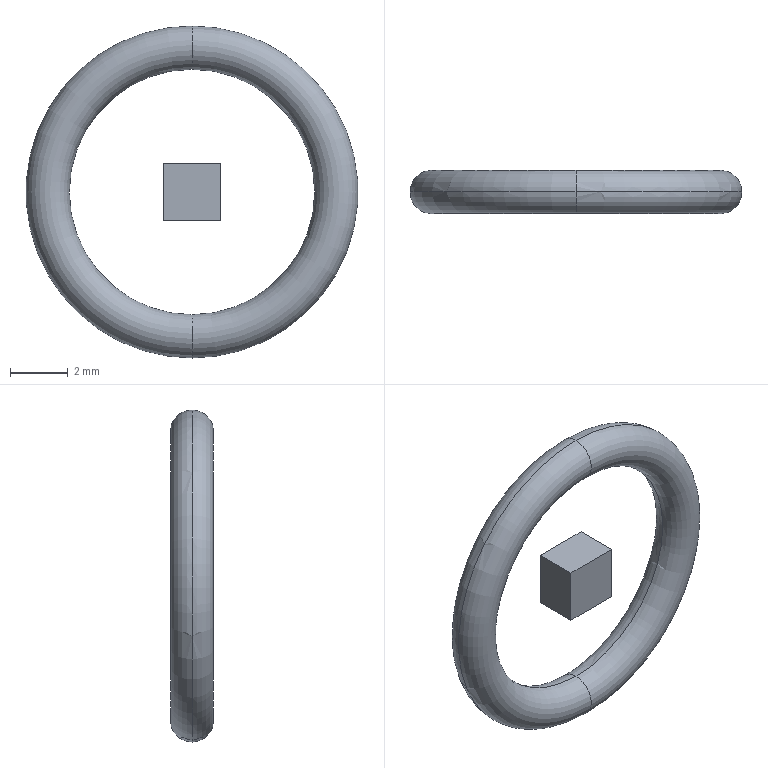Part | STEP file | O-ring ID 8.5 x 1.5 | 2 solids | 10 faces | box 11.5 x 1.5 x 11.5 mm | volume 61.517 mm3 | plane 6 | torus 4
STEP:
#1=CARTESIAN_POINT('',(0.,0.,0.));
#2=DIRECTION('',(0.,0.,1.));
#3=DIRECTION('',(1.,0.,0.));
#4=AXIS2_PLACEMENT_3D('',#1,#2,#3);
#5=CARTESIAN_POINT('',(0.,0.,5.75));
#6=VERTEX_POINT('',#5);
#7=CARTESIAN_POINT('',(0.,0.,4.25));
#8=VERTEX_POINT('',#7);
#9=CARTESIAN_POINT('',(0.,0.,5.));
#10=DIRECTION('',(1.,0.,0.));
#11=DIRECTION('',(0.,0.,-1.));
#12=AXIS2_PLACEMENT_3D('',#9,#10,#11);
#13=CIRCLE('',#12,0.75);
#14=CARTESIAN_POINT('',(0.,0.,0.));
#15=DIRECTION('',(0.,-1.,0.));
#16=DIRECTION('',(0.,0.,-1.));
#17=AXIS2_PLACEMENT_3D('',#14,#15,#16);
#18=TOROIDAL_SURFACE('',#17,5.,0.75);
#19=CARTESIAN_POINT('',(3.142,-3.142));
#20=DIRECTION('',(0.,1.));
#21=VECTOR('',#20,1.);
#22=LINE('',#19,#21);
#23=(GEOMETRIC_REPRESENTATION_CONTEXT(2)PARAMETRIC_REPRESENTATION_CONTEXT()REPRESENTATION_CONTEXT('',''));
#24=DEFINITIONAL_REPRESENTATION('',(#22),#23);
#25=PCURVE('',#18,#24);
#26=CARTESIAN_POINT('',(0.,0.,0.));
#27=DIRECTION('',(0.,-1.,0.));
#28=DIRECTION('',(0.,0.,-1.));
#29=AXIS2_PLACEMENT_3D('',#26,#27,#28);
#30=TOROIDAL_SURFACE('',#29,5.,0.75);
#31=CARTESIAN_POINT('',(3.142,-3.142));
#32=DIRECTION('',(0.,1.));
#33=VECTOR('',#32,1.);
#34=LINE('',#31,#33);
#35=(GEOMETRIC_REPRESENTATION_CONTEXT(2)PARAMETRIC_REPRESENTATION_CONTEXT()REPRESENTATION_CONTEXT('',''));
#36=DEFINITIONAL_REPRESENTATION('',(#34),#35);
#37=PCURVE('',#30,#36);
#38=SURFACE_CURVE('',#13,(#25,#37),.PCURVE_S1.);
#39=EDGE_CURVE('',#6,#8,#38,.T.);
#40=ORIENTED_EDGE('',*,*,#39,.F.);
#41=CARTESIAN_POINT('',(0.,0.,-5.75));
#42=VERTEX_POINT('',#41);
#43=CARTESIAN_POINT('',(0.,0.,0.));
#44=DIRECTION('',(0.,-1.,0.));
#45=DIRECTION('',(0.,0.,-1.));
#46=AXIS2_PLACEMENT_3D('',#43,#44,#45);
#47=CIRCLE('',#46,5.75);
#48=CARTESIAN_POINT('',(0.,0.));
#49=DIRECTION('',(1.,0.));
#50=VECTOR('',#49,1.);
#51=LINE('',#48,#50);
#52=(GEOMETRIC_REPRESENTATION_CONTEXT(2)PARAMETRIC_REPRESENTATION_CONTEXT()REPRESENTATION_CONTEXT('',''));
#53=DEFINITIONAL_REPRESENTATION('',(#51),#52);
#54=PCURVE('',#18,#53);
#55=CARTESIAN_POINT('',(0.,0.,0.));
#56=DIRECTION('',(0.,-1.,0.));
#57=DIRECTION('',(0.,0.,-1.));
#58=AXIS2_PLACEMENT_3D('',#55,#56,#57);
#59=TOROIDAL_SURFACE('',#58,5.,0.75);
#60=CARTESIAN_POINT('',(0.,6.283));
#61=DIRECTION('',(1.,0.));
#62=VECTOR('',#61,1.);
#63=LINE('',#60,#62);
#64=(GEOMETRIC_REPRESENTATION_CONTEXT(2)PARAMETRIC_REPRESENTATION_CONTEXT()REPRESENTATION_CONTEXT('',''));
#65=DEFINITIONAL_REPRESENTATION('',(#63),#64);
#66=PCURVE('',#59,#65);
#67=SURFACE_CURVE('',#47,(#54,#66),.PCURVE_S1.);
#68=EDGE_CURVE('',#6,#42,#67,.T.);
#69=ORIENTED_EDGE('',*,*,#68,.T.);
#70=CARTESIAN_POINT('',(0.,0.,-4.25));
#71=VERTEX_POINT('',#70);
#72=CARTESIAN_POINT('',(0.,0.,-5.));
#73=DIRECTION('',(-1.,0.,0.));
#74=DIRECTION('',(0.,0.,1.));
#75=AXIS2_PLACEMENT_3D('',#72,#73,#74);
#76=CIRCLE('',#75,0.75);
#77=CARTESIAN_POINT('',(6.283,-3.142));
#78=DIRECTION('',(0.,1.));
#79=VECTOR('',#78,1.);
#80=LINE('',#77,#79);
#81=(GEOMETRIC_REPRESENTATION_CONTEXT(2)PARAMETRIC_REPRESENTATION_CONTEXT()REPRESENTATION_CONTEXT('',''));
#82=DEFINITIONAL_REPRESENTATION('',(#80),#81);
#83=PCURVE('',#18,#82);
#84=CARTESIAN_POINT('',(0.,-3.142));
#85=DIRECTION('',(0.,1.));
#86=VECTOR('',#85,1.);
#87=LINE('',#84,#86);
#88=(GEOMETRIC_REPRESENTATION_CONTEXT(2)PARAMETRIC_REPRESENTATION_CONTEXT()REPRESENTATION_CONTEXT('',''));
#89=DEFINITIONAL_REPRESENTATION('',(#87),#88);
#90=PCURVE('',#30,#89);
#91=SURFACE_CURVE('',#76,(#83,#90),.PCURVE_S1.);
#92=EDGE_CURVE('',#42,#71,#91,.T.);
#93=ORIENTED_EDGE('',*,*,#92,.T.);
#94=CARTESIAN_POINT('',(0.,0.,0.));
#95=DIRECTION('',(0.,-1.,0.));
#96=DIRECTION('',(0.,0.,-1.));
#97=AXIS2_PLACEMENT_3D('',#94,#95,#96);
#98=CIRCLE('',#97,4.25);
#99=CARTESIAN_POINT('',(0.,3.142));
#100=DIRECTION('',(1.,0.));
#101=VECTOR('',#100,1.);
#102=LINE('',#99,#101);
#103=(GEOMETRIC_REPRESENTATION_CONTEXT(2)PARAMETRIC_REPRESENTATION_CONTEXT()REPRESENTATION_CONTEXT('',''));
#104=DEFINITIONAL_REPRESENTATION('',(#102),#103);
#105=PCURVE('',#18,#104);
#106=CARTESIAN_POINT('',(0.,3.142));
#107=DIRECTION('',(1.,0.));
#108=VECTOR('',#107,1.);
#109=LINE('',#106,#108);
#110=(GEOMETRIC_REPRESENTATION_CONTEXT(2)PARAMETRIC_REPRESENTATION_CONTEXT()REPRESENTATION_CONTEXT('',''));
#111=DEFINITIONAL_REPRESENTATION('',(#109),#110);
#112=PCURVE('',#59,#111);
#113=SURFACE_CURVE('',#98,(#105,#112),.PCURVE_S1.);
#114=EDGE_CURVE('',#8,#71,#113,.T.);
#115=ORIENTED_EDGE('',*,*,#114,.F.);
#116=EDGE_LOOP('',(#40,#69,#93,#115));
#117=FACE_BOUND('',#116,.T.);
#118=ADVANCED_FACE('',(#117),#18,.T.);
#119=ORIENTED_EDGE('',*,*,#92,.F.);
#120=CARTESIAN_POINT('',(0.,0.,0.));
#121=DIRECTION('',(0.,-1.,0.));
#122=DIRECTION('',(0.,0.,-1.));
#123=AXIS2_PLACEMENT_3D('',#120,#121,#122);
#124=CIRCLE('',#123,5.75);
#125=CARTESIAN_POINT('',(0.,0.));
#126=DIRECTION('',(1.,0.));
#127=VECTOR('',#126,1.);
#128=LINE('',#125,#127);
#129=(GEOMETRIC_REPRESENTATION_CONTEXT(2)PARAMETRIC_REPRESENTATION_CONTEXT()REPRESENTATION_CONTEXT('',''));
#130=DEFINITIONAL_REPRESENTATION('',(#128),#129);
#131=PCURVE('',#30,#130);
#132=CARTESIAN_POINT('',(0.,0.,0.));
#133=DIRECTION('',(0.,-1.,0.));
#134=DIRECTION('',(0.,0.,-1.));
#135=AXIS2_PLACEMENT_3D('',#132,#133,#134);
#136=TOROIDAL_SURFACE('',#135,5.,0.75);
#137=CARTESIAN_POINT('',(0.,6.283));
#138=DIRECTION('',(1.,0.));
#139=VECTOR('',#138,1.);
#140=LINE('',#137,#139);
#141=(GEOMETRIC_REPRESENTATION_CONTEXT(2)PARAMETRIC_REPRESENTATION_CONTEXT()REPRESENTATION_CONTEXT('',''));
#142=DEFINITIONAL_REPRESENTATION('',(#140),#141);
#143=PCURVE('',#136,#142);
#144=SURFACE_CURVE('',#124,(#131,#143),.PCURVE_S1.);
#145=EDGE_CURVE('',#42,#6,#144,.T.);
#146=ORIENTED_EDGE('',*,*,#145,.T.);
#147=ORIENTED_EDGE('',*,*,#39,.T.);
#148=CARTESIAN_POINT('',(0.,0.,0.));
#149=DIRECTION('',(0.,-1.,0.));
#150=DIRECTION('',(0.,0.,-1.));
#151=AXIS2_PLACEMENT_3D('',#148,#149,#150);
#152=CIRCLE('',#151,4.25);
#153=CARTESIAN_POINT('',(0.,3.142));
#154=DIRECTION('',(1.,0.));
#155=VECTOR('',#154,1.);
#156=LINE('',#153,#155);
#157=(GEOMETRIC_REPRESENTATION_CONTEXT(2)PARAMETRIC_REPRESENTATION_CONTEXT()REPRESENTATION_CONTEXT('',''));
#158=DEFINITIONAL_REPRESENTATION('',(#156),#157);
#159=PCURVE('',#30,#158);
#160=CARTESIAN_POINT('',(0.,3.142));
#161=DIRECTION('',(1.,0.));
#162=VECTOR('',#161,1.);
#163=LINE('',#160,#162);
#164=(GEOMETRIC_REPRESENTATION_CONTEXT(2)PARAMETRIC_REPRESENTATION_CONTEXT()REPRESENTATION_CONTEXT('',''));
#165=DEFINITIONAL_REPRESENTATION('',(#163),#164);
#166=PCURVE('',#136,#165);
#167=SURFACE_CURVE('',#152,(#159,#166),.PCURVE_S1.);
#168=EDGE_CURVE('',#71,#8,#167,.T.);
#169=ORIENTED_EDGE('',*,*,#168,.F.);
#170=EDGE_LOOP('',(#119,#146,#147,#169));
#171=FACE_BOUND('',#170,.T.);
#172=ADVANCED_FACE('',(#171),#30,.T.);
#173=ORIENTED_EDGE('',*,*,#145,.F.);
#174=CARTESIAN_POINT('',(0.,0.,-5.));
#175=DIRECTION('',(-1.,0.,0.));
#176=DIRECTION('',(0.,0.,1.));
#177=AXIS2_PLACEMENT_3D('',#174,#175,#176);
#178=CIRCLE('',#177,0.75);
#179=CARTESIAN_POINT('',(0.,3.142));
#180=DIRECTION('',(0.,1.));
#181=VECTOR('',#180,1.);
#182=LINE('',#179,#181);
#183=(GEOMETRIC_REPRESENTATION_CONTEXT(2)PARAMETRIC_REPRESENTATION_CONTEXT()REPRESENTATION_CONTEXT('',''));
#184=DEFINITIONAL_REPRESENTATION('',(#182),#183);
#185=PCURVE('',#136,#184);
#186=CARTESIAN_POINT('',(6.283,3.142));
#187=DIRECTION('',(0.,1.));
#188=VECTOR('',#187,1.);
#189=LINE('',#186,#188);
#190=(GEOMETRIC_REPRESENTATION_CONTEXT(2)PARAMETRIC_REPRESENTATION_CONTEXT()REPRESENTATION_CONTEXT('',''));
#191=DEFINITIONAL_REPRESENTATION('',(#189),#190);
#192=PCURVE('',#59,#191);
#193=SURFACE_CURVE('',#178,(#185,#192),.PCURVE_S1.);
#194=EDGE_CURVE('',#71,#42,#193,.T.);
#195=ORIENTED_EDGE('',*,*,#194,.F.);
#196=ORIENTED_EDGE('',*,*,#168,.T.);
#197=CARTESIAN_POINT('',(0.,0.,5.));
#198=DIRECTION('',(1.,0.,0.));
#199=DIRECTION('',(0.,0.,-1.));
#200=AXIS2_PLACEMENT_3D('',#197,#198,#199);
#201=CIRCLE('',#200,0.75);
#202=CARTESIAN_POINT('',(3.142,3.142));
#203=DIRECTION('',(0.,1.));
#204=VECTOR('',#203,1.);
#205=LINE('',#202,#204);
#206=(GEOMETRIC_REPRESENTATION_CONTEXT(2)PARAMETRIC_REPRESENTATION_CONTEXT()REPRESENTATION_CONTEXT('',''));
#207=DEFINITIONAL_REPRESENTATION('',(#205),#206);
#208=PCURVE('',#136,#207);
#209=CARTESIAN_POINT('',(3.142,3.142));
#210=DIRECTION('',(0.,1.));
#211=VECTOR('',#210,1.);
#212=LINE('',#209,#211);
#213=(GEOMETRIC_REPRESENTATION_CONTEXT(2)PARAMETRIC_REPRESENTATION_CONTEXT()REPRESENTATION_CONTEXT('',''));
#214=DEFINITIONAL_REPRESENTATION('',(#212),#213);
#215=PCURVE('',#59,#214);
#216=SURFACE_CURVE('',#201,(#208,#215),.PCURVE_S1.);
#217=EDGE_CURVE('',#8,#6,#216,.T.);
#218=ORIENTED_EDGE('',*,*,#217,.T.);
#219=EDGE_LOOP('',(#173,#195,#196,#218));
#220=FACE_BOUND('',#219,.T.);
#221=ADVANCED_FACE('',(#220),#136,.T.);
#222=ORIENTED_EDGE('',*,*,#68,.F.);
#223=ORIENTED_EDGE('',*,*,#217,.F.);
#224=ORIENTED_EDGE('',*,*,#114,.T.);
#225=ORIENTED_EDGE('',*,*,#194,.T.);
#226=EDGE_LOOP('',(#222,#223,#224,#225));
#227=FACE_BOUND('',#226,.T.);
#228=ADVANCED_FACE('',(#227),#59,.T.);
#229=CLOSED_SHELL('',(#118,#172,#221,#228));
#230=MANIFOLD_SOLID_BREP('',#229);
#231=CARTESIAN_POINT('',(1.,-0.75,1.));
#232=VERTEX_POINT('',#231);
#233=CARTESIAN_POINT('',(1.,-0.75,-1.));
#234=VERTEX_POINT('',#233);
#235=CARTESIAN_POINT('',(1.,-0.75,-1.));
#236=DIRECTION('',(0.,0.,-1.));
#237=VECTOR('',#236,1.);
#238=LINE('',#235,#237);
#239=CARTESIAN_POINT('',(1.,0.75,-1.));
#240=DIRECTION('',(-1.,0.,0.));
#241=DIRECTION('',(0.,0.,1.));
#242=AXIS2_PLACEMENT_3D('',#239,#240,#241);
#243=PLANE('',#242);
#244=CARTESIAN_POINT('',(0.,-1.5));
#245=DIRECTION('',(-1.,0.));
#246=VECTOR('',#245,1.);
#247=LINE('',#244,#246);
#248=(GEOMETRIC_REPRESENTATION_CONTEXT(2)PARAMETRIC_REPRESENTATION_CONTEXT()REPRESENTATION_CONTEXT('',''));
#249=DEFINITIONAL_REPRESENTATION('',(#247),#248);
#250=PCURVE('',#243,#249);
#251=CARTESIAN_POINT('',(0.,-0.75,0.));
#252=DIRECTION('',(0.,1.,0.));
#253=DIRECTION('',(0.,0.,1.));
#254=AXIS2_PLACEMENT_3D('',#251,#252,#253);
#255=PLANE('',#254);
#256=CARTESIAN_POINT('',(-1.,1.));
#257=DIRECTION('',(-1.,0.));
#258=VECTOR('',#257,1.);
#259=LINE('',#256,#258);
#260=(GEOMETRIC_REPRESENTATION_CONTEXT(2)PARAMETRIC_REPRESENTATION_CONTEXT()REPRESENTATION_CONTEXT('',''));
#261=DEFINITIONAL_REPRESENTATION('',(#259),#260);
#262=PCURVE('',#255,#261);
#263=SURFACE_CURVE('',#238,(#250,#262),.PCURVE_S1.);
#264=EDGE_CURVE('',#232,#234,#263,.T.);
#265=ORIENTED_EDGE('',*,*,#264,.T.);
#266=CARTESIAN_POINT('',(1.,0.75,-1.));
#267=VERTEX_POINT('',#266);
#268=CARTESIAN_POINT('',(1.,0.75,-1.));
#269=DIRECTION('',(0.,-1.,0.));
#270=VECTOR('',#269,1.);
#271=LINE('',#268,#270);
#272=CARTESIAN_POINT('',(0.,0.));
#273=DIRECTION('',(0.,-1.));
#274=VECTOR('',#273,1.);
#275=LINE('',#272,#274);
#276=(GEOMETRIC_REPRESENTATION_CONTEXT(2)PARAMETRIC_REPRESENTATION_CONTEXT()REPRESENTATION_CONTEXT('',''));
#277=DEFINITIONAL_REPRESENTATION('',(#275),#276);
#278=PCURVE('',#243,#277);
#279=CARTESIAN_POINT('',(-1.,0.75,-1.));
#280=DIRECTION('',(0.,0.,1.));
#281=DIRECTION('',(1.,0.,0.));
#282=AXIS2_PLACEMENT_3D('',#279,#280,#281);
#283=PLANE('',#282);
#284=CARTESIAN_POINT('',(2.,0.));
#285=DIRECTION('',(0.,-1.));
#286=VECTOR('',#285,1.);
#287=LINE('',#284,#286);
#288=(GEOMETRIC_REPRESENTATION_CONTEXT(2)PARAMETRIC_REPRESENTATION_CONTEXT()REPRESENTATION_CONTEXT('',''));
#289=DEFINITIONAL_REPRESENTATION('',(#287),#288);
#290=PCURVE('',#283,#289);
#291=SURFACE_CURVE('',#271,(#278,#290),.PCURVE_S1.);
#292=EDGE_CURVE('',#267,#234,#291,.T.);
#293=ORIENTED_EDGE('',*,*,#292,.F.);
#294=CARTESIAN_POINT('',(1.,0.75,1.));
#295=VERTEX_POINT('',#294);
#296=CARTESIAN_POINT('',(1.,0.75,-1.));
#297=DIRECTION('',(0.,0.,-1.));
#298=VECTOR('',#297,1.);
#299=LINE('',#296,#298);
#300=CARTESIAN_POINT('',(0.,0.));
#301=DIRECTION('',(-1.,0.));
#302=VECTOR('',#301,1.);
#303=LINE('',#300,#302);
#304=(GEOMETRIC_REPRESENTATION_CONTEXT(2)PARAMETRIC_REPRESENTATION_CONTEXT()REPRESENTATION_CONTEXT('',''));
#305=DEFINITIONAL_REPRESENTATION('',(#303),#304);
#306=PCURVE('',#243,#305);
#307=CARTESIAN_POINT('',(0.,0.75,0.));
#308=DIRECTION('',(0.,1.,0.));
#309=DIRECTION('',(0.,0.,1.));
#310=AXIS2_PLACEMENT_3D('',#307,#308,#309);
#311=PLANE('',#310);
#312=CARTESIAN_POINT('',(-1.,1.));
#313=DIRECTION('',(-1.,0.));
#314=VECTOR('',#313,1.);
#315=LINE('',#312,#314);
#316=(GEOMETRIC_REPRESENTATION_CONTEXT(2)PARAMETRIC_REPRESENTATION_CONTEXT()REPRESENTATION_CONTEXT('',''));
#317=DEFINITIONAL_REPRESENTATION('',(#315),#316);
#318=PCURVE('',#311,#317);
#319=SURFACE_CURVE('',#299,(#306,#318),.PCURVE_S1.);
#320=EDGE_CURVE('',#295,#267,#319,.T.);
#321=ORIENTED_EDGE('',*,*,#320,.F.);
#322=CARTESIAN_POINT('',(1.,0.75,1.));
#323=DIRECTION('',(0.,-1.,0.));
#324=VECTOR('',#323,1.);
#325=LINE('',#322,#324);
#326=CARTESIAN_POINT('',(2.,0.));
#327=DIRECTION('',(0.,-1.));
#328=VECTOR('',#327,1.);
#329=LINE('',#326,#328);
#330=(GEOMETRIC_REPRESENTATION_CONTEXT(2)PARAMETRIC_REPRESENTATION_CONTEXT()REPRESENTATION_CONTEXT('',''));
#331=DEFINITIONAL_REPRESENTATION('',(#329),#330);
#332=PCURVE('',#243,#331);
#333=CARTESIAN_POINT('',(-1.,0.75,1.));
#334=DIRECTION('',(0.,0.,-1.));
#335=DIRECTION('',(-1.,0.,0.));
#336=AXIS2_PLACEMENT_3D('',#333,#334,#335);
#337=PLANE('',#336);
#338=CARTESIAN_POINT('',(-2.,0.));
#339=DIRECTION('',(0.,-1.));
#340=VECTOR('',#339,1.);
#341=LINE('',#338,#340);
#342=(GEOMETRIC_REPRESENTATION_CONTEXT(2)PARAMETRIC_REPRESENTATION_CONTEXT()REPRESENTATION_CONTEXT('',''));
#343=DEFINITIONAL_REPRESENTATION('',(#341),#342);
#344=PCURVE('',#337,#343);
#345=SURFACE_CURVE('',#325,(#332,#344),.PCURVE_S1.);
#346=EDGE_CURVE('',#295,#232,#345,.T.);
#347=ORIENTED_EDGE('',*,*,#346,.T.);
#348=EDGE_LOOP('',(#265,#293,#321,#347));
#349=FACE_BOUND('',#348,.T.);
#350=ADVANCED_FACE('',(#349),#243,.F.);
#351=CARTESIAN_POINT('',(-1.,-0.75,-1.));
#352=VERTEX_POINT('',#351);
#353=CARTESIAN_POINT('',(-1.,-0.75,-1.));
#354=DIRECTION('',(-1.,0.,0.));
#355=VECTOR('',#354,1.);
#356=LINE('',#353,#355);
#357=CARTESIAN_POINT('',(0.,-1.5));
#358=DIRECTION('',(-1.,0.));
#359=VECTOR('',#358,1.);
#360=LINE('',#357,#359);
#361=(GEOMETRIC_REPRESENTATION_CONTEXT(2)PARAMETRIC_REPRESENTATION_CONTEXT()REPRESENTATION_CONTEXT('',''));
#362=DEFINITIONAL_REPRESENTATION('',(#360),#361);
#363=PCURVE('',#283,#362);
#364=CARTESIAN_POINT('',(-1.,-1.));
#365=DIRECTION('',(0.,-1.));
#366=VECTOR('',#365,1.);
#367=LINE('',#364,#366);
#368=(GEOMETRIC_REPRESENTATION_CONTEXT(2)PARAMETRIC_REPRESENTATION_CONTEXT()REPRESENTATION_CONTEXT('',''));
#369=DEFINITIONAL_REPRESENTATION('',(#367),#368);
#370=PCURVE('',#255,#369);
#371=SURFACE_CURVE('',#356,(#363,#370),.PCURVE_S1.);
#372=EDGE_CURVE('',#234,#352,#371,.T.);
#373=ORIENTED_EDGE('',*,*,#372,.T.);
#374=CARTESIAN_POINT('',(-1.,0.75,-1.));
#375=VERTEX_POINT('',#374);
#376=CARTESIAN_POINT('',(-1.,0.75,-1.));
#377=DIRECTION('',(0.,-1.,0.));
#378=VECTOR('',#377,1.);
#379=LINE('',#376,#378);
#380=CARTESIAN_POINT('',(0.,0.));
#381=DIRECTION('',(0.,-1.));
#382=VECTOR('',#381,1.);
#383=LINE('',#380,#382);
#384=(GEOMETRIC_REPRESENTATION_CONTEXT(2)PARAMETRIC_REPRESENTATION_CONTEXT()REPRESENTATION_CONTEXT('',''));
#385=DEFINITIONAL_REPRESENTATION('',(#383),#384);
#386=PCURVE('',#283,#385);
#387=CARTESIAN_POINT('',(-1.,0.75,-1.));
#388=DIRECTION('',(1.,0.,0.));
#389=DIRECTION('',(0.,0.,-1.));
#390=AXIS2_PLACEMENT_3D('',#387,#388,#389);
#391=PLANE('',#390);
#392=CARTESIAN_POINT('',(0.,0.));
#393=DIRECTION('',(0.,-1.));
#394=VECTOR('',#393,1.);
#395=LINE('',#392,#394);
#396=(GEOMETRIC_REPRESENTATION_CONTEXT(2)PARAMETRIC_REPRESENTATION_CONTEXT()REPRESENTATION_CONTEXT('',''));
#397=DEFINITIONAL_REPRESENTATION('',(#395),#396);
#398=PCURVE('',#391,#397);
#399=SURFACE_CURVE('',#379,(#386,#398),.PCURVE_S1.);
#400=EDGE_CURVE('',#375,#352,#399,.T.);
#401=ORIENTED_EDGE('',*,*,#400,.F.);
#402=CARTESIAN_POINT('',(-1.,0.75,-1.));
#403=DIRECTION('',(-1.,0.,0.));
#404=VECTOR('',#403,1.);
#405=LINE('',#402,#404);
#406=CARTESIAN_POINT('',(0.,0.));
#407=DIRECTION('',(-1.,0.));
#408=VECTOR('',#407,1.);
#409=LINE('',#406,#408);
#410=(GEOMETRIC_REPRESENTATION_CONTEXT(2)PARAMETRIC_REPRESENTATION_CONTEXT()REPRESENTATION_CONTEXT('',''));
#411=DEFINITIONAL_REPRESENTATION('',(#409),#410);
#412=PCURVE('',#283,#411);
#413=CARTESIAN_POINT('',(-1.,-1.));
#414=DIRECTION('',(0.,-1.));
#415=VECTOR('',#414,1.);
#416=LINE('',#413,#415);
#417=(GEOMETRIC_REPRESENTATION_CONTEXT(2)PARAMETRIC_REPRESENTATION_CONTEXT()REPRESENTATION_CONTEXT('',''));
#418=DEFINITIONAL_REPRESENTATION('',(#416),#417);
#419=PCURVE('',#311,#418);
#420=SURFACE_CURVE('',#405,(#412,#419),.PCURVE_S1.);
#421=EDGE_CURVE('',#267,#375,#420,.T.);
#422=ORIENTED_EDGE('',*,*,#421,.F.);
#423=ORIENTED_EDGE('',*,*,#292,.T.);
#424=EDGE_LOOP('',(#373,#401,#422,#423));
#425=FACE_BOUND('',#424,.T.);
#426=ADVANCED_FACE('',(#425),#283,.F.);
#427=CARTESIAN_POINT('',(-1.,-0.75,1.));
#428=VERTEX_POINT('',#427);
#429=CARTESIAN_POINT('',(-1.,-0.75,-1.));
#430=DIRECTION('',(0.,0.,1.));
#431=VECTOR('',#430,1.);
#432=LINE('',#429,#431);
#433=CARTESIAN_POINT('',(0.,-1.5));
#434=DIRECTION('',(-1.,0.));
#435=VECTOR('',#434,1.);
#436=LINE('',#433,#435);
#437=(GEOMETRIC_REPRESENTATION_CONTEXT(2)PARAMETRIC_REPRESENTATION_CONTEXT()REPRESENTATION_CONTEXT('',''));
#438=DEFINITIONAL_REPRESENTATION('',(#436),#437);
#439=PCURVE('',#391,#438);
#440=CARTESIAN_POINT('',(-1.,-1.));
#441=DIRECTION('',(1.,0.));
#442=VECTOR('',#441,1.);
#443=LINE('',#440,#442);
#444=(GEOMETRIC_REPRESENTATION_CONTEXT(2)PARAMETRIC_REPRESENTATION_CONTEXT()REPRESENTATION_CONTEXT('',''));
#445=DEFINITIONAL_REPRESENTATION('',(#443),#444);
#446=PCURVE('',#255,#445);
#447=SURFACE_CURVE('',#432,(#439,#446),.PCURVE_S1.);
#448=EDGE_CURVE('',#352,#428,#447,.T.);
#449=ORIENTED_EDGE('',*,*,#448,.T.);
#450=CARTESIAN_POINT('',(-1.,0.75,1.));
#451=VERTEX_POINT('',#450);
#452=CARTESIAN_POINT('',(-1.,0.75,1.));
#453=DIRECTION('',(0.,-1.,0.));
#454=VECTOR('',#453,1.);
#455=LINE('',#452,#454);
#456=CARTESIAN_POINT('',(-2.,0.));
#457=DIRECTION('',(0.,-1.));
#458=VECTOR('',#457,1.);
#459=LINE('',#456,#458);
#460=(GEOMETRIC_REPRESENTATION_CONTEXT(2)PARAMETRIC_REPRESENTATION_CONTEXT()REPRESENTATION_CONTEXT('',''));
#461=DEFINITIONAL_REPRESENTATION('',(#459),#460);
#462=PCURVE('',#391,#461);
#463=CARTESIAN_POINT('',(0.,0.));
#464=DIRECTION('',(0.,-1.));
#465=VECTOR('',#464,1.);
#466=LINE('',#463,#465);
#467=(GEOMETRIC_REPRESENTATION_CONTEXT(2)PARAMETRIC_REPRESENTATION_CONTEXT()REPRESENTATION_CONTEXT('',''));
#468=DEFINITIONAL_REPRESENTATION('',(#466),#467);
#469=PCURVE('',#337,#468);
#470=SURFACE_CURVE('',#455,(#462,#469),.PCURVE_S1.);
#471=EDGE_CURVE('',#451,#428,#470,.T.);
#472=ORIENTED_EDGE('',*,*,#471,.F.);
#473=CARTESIAN_POINT('',(-1.,0.75,-1.));
#474=DIRECTION('',(0.,0.,1.));
#475=VECTOR('',#474,1.);
#476=LINE('',#473,#475);
#477=CARTESIAN_POINT('',(0.,0.));
#478=DIRECTION('',(-1.,0.));
#479=VECTOR('',#478,1.);
#480=LINE('',#477,#479);
#481=(GEOMETRIC_REPRESENTATION_CONTEXT(2)PARAMETRIC_REPRESENTATION_CONTEXT()REPRESENTATION_CONTEXT('',''));
#482=DEFINITIONAL_REPRESENTATION('',(#480),#481);
#483=PCURVE('',#391,#482);
#484=CARTESIAN_POINT('',(-1.,-1.));
#485=DIRECTION('',(1.,0.));
#486=VECTOR('',#485,1.);
#487=LINE('',#484,#486);
#488=(GEOMETRIC_REPRESENTATION_CONTEXT(2)PARAMETRIC_REPRESENTATION_CONTEXT()REPRESENTATION_CONTEXT('',''));
#489=DEFINITIONAL_REPRESENTATION('',(#487),#488);
#490=PCURVE('',#311,#489);
#491=SURFACE_CURVE('',#476,(#483,#490),.PCURVE_S1.);
#492=EDGE_CURVE('',#375,#451,#491,.T.);
#493=ORIENTED_EDGE('',*,*,#492,.F.);
#494=ORIENTED_EDGE('',*,*,#400,.T.);
#495=EDGE_LOOP('',(#449,#472,#493,#494));
#496=FACE_BOUND('',#495,.T.);
#497=ADVANCED_FACE('',(#496),#391,.F.);
#498=CARTESIAN_POINT('',(-1.,-0.75,1.));
#499=DIRECTION('',(1.,0.,0.));
#500=VECTOR('',#499,1.);
#501=LINE('',#498,#500);
#502=CARTESIAN_POINT('',(0.,-1.5));
#503=DIRECTION('',(-1.,0.));
#504=VECTOR('',#503,1.);
#505=LINE('',#502,#504);
#506=(GEOMETRIC_REPRESENTATION_CONTEXT(2)PARAMETRIC_REPRESENTATION_CONTEXT()REPRESENTATION_CONTEXT('',''));
#507=DEFINITIONAL_REPRESENTATION('',(#505),#506);
#508=PCURVE('',#337,#507);
#509=CARTESIAN_POINT('',(1.,-1.));
#510=DIRECTION('',(0.,1.));
#511=VECTOR('',#510,1.);
#512=LINE('',#509,#511);
#513=(GEOMETRIC_REPRESENTATION_CONTEXT(2)PARAMETRIC_REPRESENTATION_CONTEXT()REPRESENTATION_CONTEXT('',''));
#514=DEFINITIONAL_REPRESENTATION('',(#512),#513);
#515=PCURVE('',#255,#514);
#516=SURFACE_CURVE('',#501,(#508,#515),.PCURVE_S1.);
#517=EDGE_CURVE('',#428,#232,#516,.T.);
#518=ORIENTED_EDGE('',*,*,#517,.T.);
#519=ORIENTED_EDGE('',*,*,#346,.F.);
#520=CARTESIAN_POINT('',(-1.,0.75,1.));
#521=DIRECTION('',(1.,0.,0.));
#522=VECTOR('',#521,1.);
#523=LINE('',#520,#522);
#524=CARTESIAN_POINT('',(0.,0.));
#525=DIRECTION('',(-1.,0.));
#526=VECTOR('',#525,1.);
#527=LINE('',#524,#526);
#528=(GEOMETRIC_REPRESENTATION_CONTEXT(2)PARAMETRIC_REPRESENTATION_CONTEXT()REPRESENTATION_CONTEXT('',''));
#529=DEFINITIONAL_REPRESENTATION('',(#527),#528);
#530=PCURVE('',#337,#529);
#531=CARTESIAN_POINT('',(1.,-1.));
#532=DIRECTION('',(0.,1.));
#533=VECTOR('',#532,1.);
#534=LINE('',#531,#533);
#535=(GEOMETRIC_REPRESENTATION_CONTEXT(2)PARAMETRIC_REPRESENTATION_CONTEXT()REPRESENTATION_CONTEXT('',''));
#536=DEFINITIONAL_REPRESENTATION('',(#534),#535);
#537=PCURVE('',#311,#536);
#538=SURFACE_CURVE('',#523,(#530,#537),.PCURVE_S1.);
#539=EDGE_CURVE('',#451,#295,#538,.T.);
#540=ORIENTED_EDGE('',*,*,#539,.F.);
#541=ORIENTED_EDGE('',*,*,#471,.T.);
#542=EDGE_LOOP('',(#518,#519,#540,#541));
#543=FACE_BOUND('',#542,.T.);
#544=ADVANCED_FACE('',(#543),#337,.F.);
#545=ORIENTED_EDGE('',*,*,#320,.T.);
#546=ORIENTED_EDGE('',*,*,#421,.T.);
#547=ORIENTED_EDGE('',*,*,#492,.T.);
#548=ORIENTED_EDGE('',*,*,#539,.T.);
#549=EDGE_LOOP('',(#545,#546,#547,#548));
#550=FACE_BOUND('',#549,.T.);
#551=ADVANCED_FACE('',(#550),#311,.T.);
#552=ORIENTED_EDGE('',*,*,#264,.F.);
#553=ORIENTED_EDGE('',*,*,#517,.F.);
#554=ORIENTED_EDGE('',*,*,#448,.F.);
#555=ORIENTED_EDGE('',*,*,#372,.F.);
#556=EDGE_LOOP('',(#552,#553,#554,#555));
#557=FACE_BOUND('',#556,.T.);
#558=ADVANCED_FACE('',(#557),#255,.F.);
#559=CLOSED_SHELL('',(#350,#426,#497,#544,#551,#558));
#560=MANIFOLD_SOLID_BREP('',#559);
#561=(LENGTH_UNIT()NAMED_UNIT(*)SI_UNIT(.MILLI.,.METRE.));
#562=UNCERTAINTY_MEASURE_WITH_UNIT(LENGTH_MEASURE(0.0000001),#561,'','');
#563=(NAMED_UNIT(*)PLANE_ANGLE_UNIT()SI_UNIT($,.RADIAN.));
#564=(NAMED_UNIT(*)SI_UNIT($,.STERADIAN.)SOLID_ANGLE_UNIT());
#565=(GEOMETRIC_REPRESENTATION_CONTEXT(3)GLOBAL_UNCERTAINTY_ASSIGNED_CONTEXT((#562))GLOBAL_UNIT_ASSIGNED_CONTEXT((#561,#563,#564))REPRESENTATION_CONTEXT('',''));
#566=SHAPE_REPRESENTATION('',(#4,#230,#560),#565);